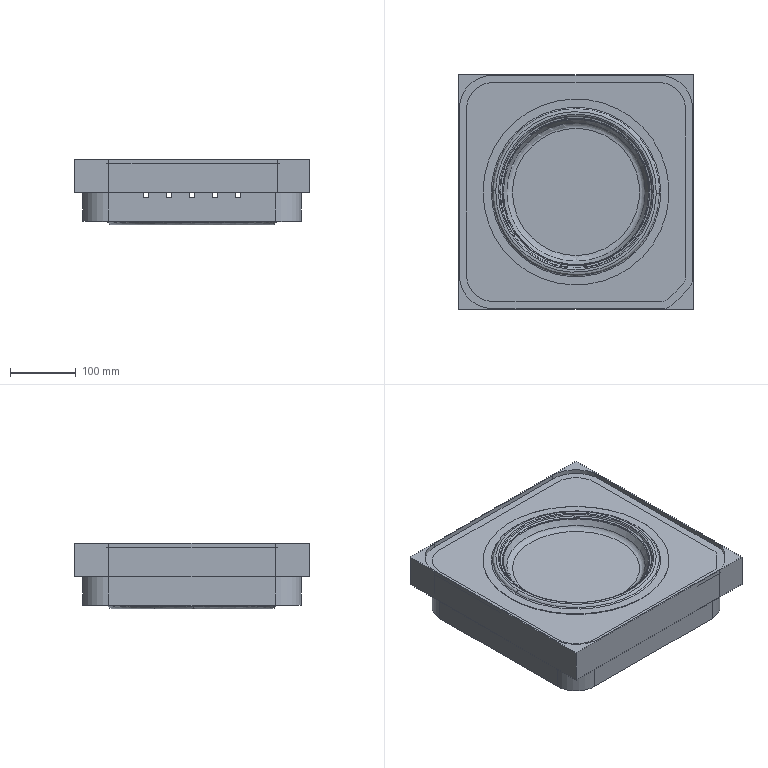NC program | NX | posted with a generic post | part box 356 x 356 x 99.5 mm
Lines 142662 to 142759 of 165566:
(DRILLING , TOOL : V2.0)
N285298 M6
N285300 G53
N285302 G17 G0 G90 X-48.846 Y-122.012 S2000 M3 M8
N285304 G43 Z200.5 H0
N285306 G94 G81 G98 Z42.725 F150. R47.725
N285308 X-24.873 Y-129.051
N285310 X0. Y-131.426
N285312 X24.873 Y-129.051
N285314 X48.846 Y-122.012
N285316 X71.054 Y-110.563
N285318 X90.695 Y-95.118
N285320 X107.057 Y-76.235
N285322 X119.55 Y-54.597
N285324 X127.722 Y-30.985
N285326 X131.278 Y-6.254
N285328 X130.089 Y18.704
N285330 X124.198 Y42.985
N285332 X113.819 Y65.713
N285334 X99.326 Y86.066
N285336 X81.242 Y103.308
N285338 X60.223 Y116.816
N285340 X37.027 Y126.103
N285342 X12.493 Y130.831
N285344 X-12.493
N285346 X-37.027 Y126.103
N285348 X-60.223 Y116.816
N285350 X-81.242 Y103.308
N285352 X-99.325 Y86.066
N285354 X-113.818 Y65.713
N285356 X-124.198 Y42.986
N285358 X-130.088 Y18.704
N285360 X-131.277 Y-6.253
N285362 X-127.722 Y-30.985
N285364 X-119.55 Y-54.596
N285366 X-107.057 Y-76.235
N285368 X-90.695 Y-95.118
N285370 X-71.054 Y-110.563
N285372 X-48.53 Y-79.804 Z27.72 R32.72
N285374 X-68.261 Y-63.751
N285376 X-82.929 Y-42.971
N285378 X-91.447 Y-19.003
N285380 X-93.183 Y6.374
N285382 X-88.008 Y31.278
N285384 X-76.306 Y53.863
N285386 X-54.585 Y41.221
N285388 X-36.009 Y58.156
N285390 X-25.511 Y35.112
N285392 X0. Y43.401
N285394 Y18.401
N285396 X18.401 Y0.
N285398 X0. Y-18.401
N285400 X-18.401 Y0.
N285402 X-41.277 Y-13.412
N285404 Y13.412
N285406 X-65.79 Y18.719
N285408 X-68.109 Y-6.311
N285410 X-61.23 Y-30.489
N285412 X-46.081 Y-50.549
N285414 X-25.511 Y-35.112
N285416 X0. Y-43.401
N285418 X25.511 Y-35.112
N285420 X41.277 Y-13.412
N285422 Y13.412
N285424 X25.511 Y35.112
N285426 X36.009 Y58.156
N285428 X54.585 Y41.221
N285430 X65.79 Y18.719
N285432 X68.109 Y-6.311
N285434 X61.23 Y-30.489
N285436 X46.081 Y-50.549
N285438 X24.709 Y-63.782
N285440 X0. Y-68.401
N285442 X-24.709 Y-63.782
N285444 X-25.199 Y-89.937
N285446 X0. Y-93.401
N285448 X25.199 Y-89.937
N285450 X48.53 Y-79.804
N285452 X68.261 Y-63.751
N285454 X82.929 Y-42.971
N285456 X91.447 Y-19.003
N285458 X93.183 Y6.374
N285460 X88.008 Y31.278
N285462 X76.306 Y53.863
N285464 X58.944 Y72.452
N285466 X37.211 Y85.669
N285468 X12.718 Y92.531
N285470 X12.569 Y67.236
N285472 X-12.569
N285474 X-12.718 Y92.531
N285476 X-37.211 Y85.669
N285478 X-58.944 Y72.452
N285480 G80
N285482 G0 X-58.944 Y72.452 Z200.5
N285484 M9
N285486 M5